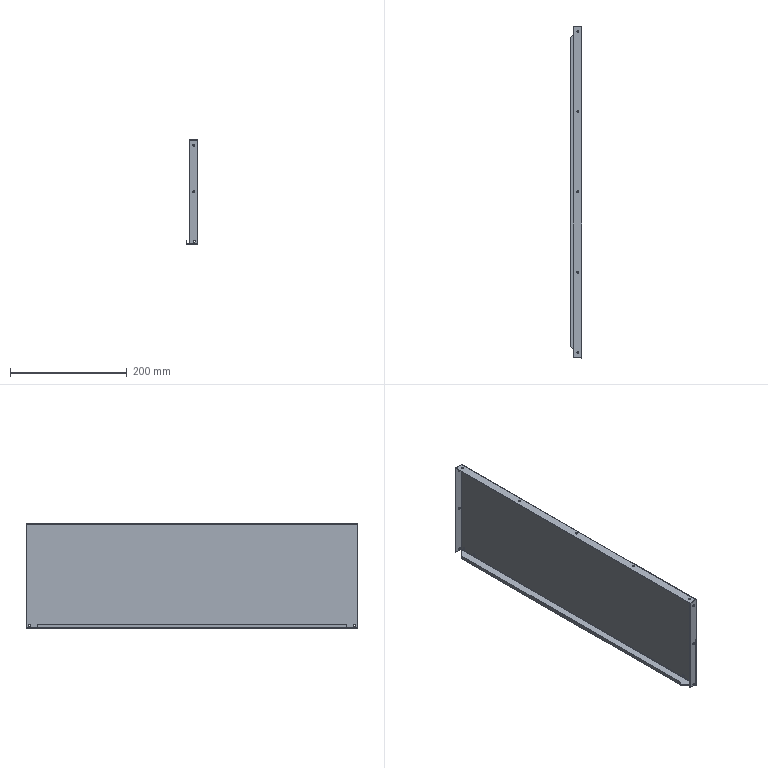Part | SolidWorks | features BaseBody 1 | 1 solid | 78 faces | box 19.9 x 568.8 x 179.4 mm | volume 76913 mm3 | cylinder 40 | plane 32 | spline 6 | commonest cylinder face diameters 3.5 x30 0.4 x5 1.6 x5